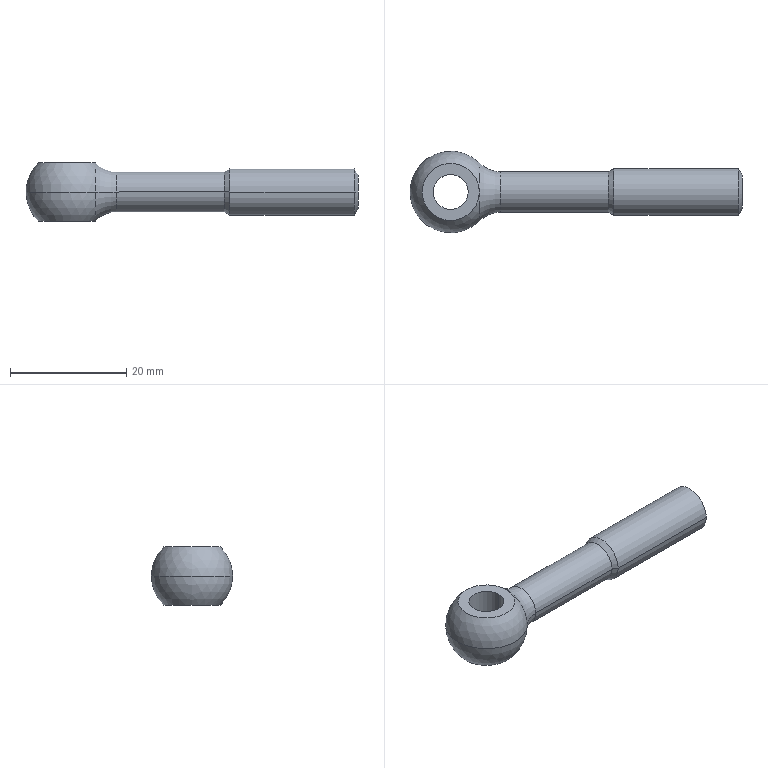Part | SolidWorks | features Cut 2, Revolution 2, Chamfer 1, Fillet 1, LPattern 1, RevCut 1 | 1 solid | 17 faces | box 57 x 14 x 10 mm | volume 2922 mm3 | cylinder 6 | cone 4 | plane 3 | torus 2 | sphere 2 | commonest cylinder face diameters 6 x2 6.918 x2 8 x2
STEP:
#1=CARTESIAN_POINT('',(4.965,4.934,0.));
#2=VERTEX_POINT('',#1);
#3=CARTESIAN_POINT('',(4.965,-4.934,0.));
#4=VERTEX_POINT('',#3);
#5=CARTESIAN_POINT('',(4.965,0.,0.));
#6=DIRECTION('',(-1.,0.,0.));
#7=DIRECTION('',(0.,-1.,0.));
#8=AXIS2_PLACEMENT_3D('',#5,#6,#7);
#9=CIRCLE('',#8,4.934);
#10=EDGE_CURVE('',#2,#4,#9,.T.);
#11=ORIENTED_EDGE('',*,*,#10,.F.);
#12=CARTESIAN_POINT('',(8.512,3.459,0.));
#13=VERTEX_POINT('',#12);
#14=CARTESIAN_POINT('',(8.512,8.459,0.));
#15=DIRECTION('',(0.,0.,1.));
#16=DIRECTION('',(0.,-1.,0.));
#17=AXIS2_PLACEMENT_3D('',#14,#15,#16);
#18=CIRCLE('',#17,5.);
#19=EDGE_CURVE('',#2,#13,#18,.T.);
#20=ORIENTED_EDGE('',*,*,#19,.T.);
#21=CARTESIAN_POINT('',(8.512,-3.459,0.));
#22=VERTEX_POINT('',#21);
#23=CARTESIAN_POINT('',(8.512,0.,0.));
#24=DIRECTION('',(1.,0.,0.));
#25=DIRECTION('',(0.,-1.,0.));
#26=AXIS2_PLACEMENT_3D('',#23,#24,#25);
#27=CIRCLE('',#26,3.459);
#28=EDGE_CURVE('',#22,#13,#27,.T.);
#29=ORIENTED_EDGE('',*,*,#28,.F.);
#30=CARTESIAN_POINT('',(8.512,-8.459,0.));
#31=DIRECTION('',(0.,0.,-1.));
#32=DIRECTION('',(-1.,0.,0.));
#33=AXIS2_PLACEMENT_3D('',#30,#31,#32);
#34=CIRCLE('',#33,5.);
#35=EDGE_CURVE('',#4,#22,#34,.T.);
#36=ORIENTED_EDGE('',*,*,#35,.F.);
#37=EDGE_LOOP('',(#11,#20,#29,#36));
#38=FACE_OUTER_BOUND('',#37,.T.);
#39=CARTESIAN_POINT('',(8.512,0.,0.));
#40=DIRECTION('',(-1.,0.,0.));
#41=DIRECTION('',(0.,-1.,0.));
#42=AXIS2_PLACEMENT_3D('',#39,#40,#41);
#43=TOROIDAL_SURFACE('',#42,8.459,5.);
#44=ADVANCED_FACE('',(#38),#43,.F.);
#45=CARTESIAN_POINT('',(50.,-2.918,0.));
#46=VERTEX_POINT('',#45);
#47=CARTESIAN_POINT('',(50.,2.917,0.));
#48=VERTEX_POINT('',#47);
#49=CARTESIAN_POINT('',(50.,0.,0.));
#50=DIRECTION('',(-1.,0.,0.));
#51=DIRECTION('',(0.,-1.,0.));
#52=AXIS2_PLACEMENT_3D('',#49,#50,#51);
#53=CIRCLE('',#52,2.918);
#54=EDGE_CURVE('',#46,#48,#53,.T.);
#55=ORIENTED_EDGE('',*,*,#54,.T.);
#56=CARTESIAN_POINT('',(49.375,4.,0.));
#57=VERTEX_POINT('',#56);
#58=CARTESIAN_POINT('',(49.375,4.,0.));
#59=DIRECTION('',(-0.5,0.866,0.));
#60=VECTOR('',#59,1000.);
#61=LINE('',#58,#60);
#62=EDGE_CURVE('',#48,#57,#61,.T.);
#63=ORIENTED_EDGE('',*,*,#62,.T.);
#64=CARTESIAN_POINT('',(49.375,-4.,0.));
#65=VERTEX_POINT('',#64);
#66=CARTESIAN_POINT('',(49.375,0.,0.));
#67=DIRECTION('',(-1.,0.,0.));
#68=DIRECTION('',(0.,-1.,0.));
#69=AXIS2_PLACEMENT_3D('',#66,#67,#68);
#70=CIRCLE('',#69,4.);
#71=EDGE_CURVE('',#65,#57,#70,.T.);
#72=ORIENTED_EDGE('',*,*,#71,.F.);
#73=CARTESIAN_POINT('',(49.375,-4.,0.));
#74=DIRECTION('',(-0.5,-0.866,0.));
#75=VECTOR('',#74,1000.);
#76=LINE('',#73,#75);
#77=EDGE_CURVE('',#46,#65,#76,.T.);
#78=ORIENTED_EDGE('',*,*,#77,.F.);
#79=EDGE_LOOP('',(#55,#63,#72,#78));
#80=FACE_OUTER_BOUND('',#79,.T.);
#81=CARTESIAN_POINT('',(49.375,0.,0.));
#82=DIRECTION('',(-1.,0.,0.));
#83=DIRECTION('',(0.,-1.,0.));
#84=AXIS2_PLACEMENT_3D('',#81,#82,#83);
#85=CONICAL_SURFACE('',#84,4.,1.047);
#86=ADVANCED_FACE('',(#80),#85,.T.);
#87=CARTESIAN_POINT('',(27.063,-3.459,0.));
#88=VERTEX_POINT('',#87);
#89=CARTESIAN_POINT('',(27.063,3.459,0.));
#90=VERTEX_POINT('',#89);
#91=CARTESIAN_POINT('',(27.063,0.,0.));
#92=DIRECTION('',(-1.,0.,0.));
#93=DIRECTION('',(0.,-1.,0.));
#94=AXIS2_PLACEMENT_3D('',#91,#92,#93);
#95=CIRCLE('',#94,3.459);
#96=EDGE_CURVE('',#88,#90,#95,.T.);
#97=ORIENTED_EDGE('',*,*,#96,.F.);
#98=CARTESIAN_POINT('',(28.,-4.,0.));
#99=VERTEX_POINT('',#98);
#100=CARTESIAN_POINT('',(28.,-4.,0.));
#101=DIRECTION('',(0.866,-0.5,0.));
#102=VECTOR('',#101,1000.);
#103=LINE('',#100,#102);
#104=EDGE_CURVE('',#88,#99,#103,.T.);
#105=ORIENTED_EDGE('',*,*,#104,.T.);
#106=CARTESIAN_POINT('',(28.,4.,0.));
#107=VERTEX_POINT('',#106);
#108=CARTESIAN_POINT('',(28.,0.,0.));
#109=DIRECTION('',(-1.,0.,0.));
#110=DIRECTION('',(0.,-1.,0.));
#111=AXIS2_PLACEMENT_3D('',#108,#109,#110);
#112=CIRCLE('',#111,4.);
#113=EDGE_CURVE('',#99,#107,#112,.T.);
#114=ORIENTED_EDGE('',*,*,#113,.T.);
#115=CARTESIAN_POINT('',(28.,4.,0.));
#116=DIRECTION('',(0.866,0.5,0.));
#117=VECTOR('',#116,1000.);
#118=LINE('',#115,#117);
#119=EDGE_CURVE('',#90,#107,#118,.T.);
#120=ORIENTED_EDGE('',*,*,#119,.F.);
#121=EDGE_LOOP('',(#97,#105,#114,#120));
#122=FACE_OUTER_BOUND('',#121,.T.);
#123=CARTESIAN_POINT('',(28.,0.,0.));
#124=DIRECTION('',(1.,0.,0.));
#125=DIRECTION('',(0.,1.,0.));
#126=AXIS2_PLACEMENT_3D('',#123,#124,#125);
#127=CONICAL_SURFACE('',#126,4.,0.5236);
#128=ADVANCED_FACE('',(#122),#127,.T.);
#129=ORIENTED_EDGE('',*,*,#96,.T.);
#130=CARTESIAN_POINT('',(0.,3.459,0.));
#131=DIRECTION('',(-1.,0.,0.));
#132=VECTOR('',#131,1000.);
#133=LINE('',#130,#132);
#134=EDGE_CURVE('',#90,#13,#133,.T.);
#135=ORIENTED_EDGE('',*,*,#134,.T.);
#136=CARTESIAN_POINT('',(8.512,0.,0.));
#137=DIRECTION('',(1.,0.,0.));
#138=DIRECTION('',(0.,-1.,0.));
#139=AXIS2_PLACEMENT_3D('',#136,#137,#138);
#140=CIRCLE('',#139,3.459);
#141=EDGE_CURVE('',#13,#22,#140,.T.);
#142=ORIENTED_EDGE('',*,*,#141,.T.);
#143=CARTESIAN_POINT('',(0.,-3.459,0.));
#144=DIRECTION('',(-1.,0.,0.));
#145=VECTOR('',#144,1000.);
#146=LINE('',#143,#145);
#147=EDGE_CURVE('',#88,#22,#146,.T.);
#148=ORIENTED_EDGE('',*,*,#147,.F.);
#149=EDGE_LOOP('',(#129,#135,#142,#148));
#150=FACE_OUTER_BOUND('',#149,.T.);
#151=CARTESIAN_POINT('',(0.,0.,0.));
#152=DIRECTION('',(-1.,0.,0.));
#153=DIRECTION('',(0.,-1.,0.));
#154=AXIS2_PLACEMENT_3D('',#151,#152,#153);
#155=CYLINDRICAL_SURFACE('',#154,3.459);
#156=ADVANCED_FACE('',(#150),#155,.T.);
#157=CARTESIAN_POINT('',(-3.,0.,-5.));
#158=VERTEX_POINT('',#157);
#159=CARTESIAN_POINT('',(3.,0.,-5.));
#160=VERTEX_POINT('',#159);
#161=CARTESIAN_POINT('',(0.,0.,-5.));
#162=DIRECTION('',(0.,0.,1.));
#163=DIRECTION('',(1.,0.,0.));
#164=AXIS2_PLACEMENT_3D('',#161,#162,#163);
#165=CIRCLE('',#164,3.);
#166=EDGE_CURVE('',#158,#160,#165,.T.);
#167=ORIENTED_EDGE('',*,*,#166,.F.);
#168=CARTESIAN_POINT('',(-3.,0.,5.));
#169=VERTEX_POINT('',#168);
#170=CARTESIAN_POINT('',(-3.,0.,-5.));
#171=DIRECTION('',(0.,0.,1.));
#172=VECTOR('',#171,1000.);
#173=LINE('',#170,#172);
#174=EDGE_CURVE('',#158,#169,#173,.T.);
#175=ORIENTED_EDGE('',*,*,#174,.T.);
#176=CARTESIAN_POINT('',(3.,0.,5.));
#177=VERTEX_POINT('',#176);
#178=CARTESIAN_POINT('',(0.,0.,5.));
#179=DIRECTION('',(0.,0.,1.));
#180=DIRECTION('',(1.,0.,0.));
#181=AXIS2_PLACEMENT_3D('',#178,#179,#180);
#182=CIRCLE('',#181,3.);
#183=EDGE_CURVE('',#169,#177,#182,.T.);
#184=ORIENTED_EDGE('',*,*,#183,.T.);
#185=CARTESIAN_POINT('',(3.,0.,-5.));
#186=DIRECTION('',(0.,0.,1.));
#187=VECTOR('',#186,1000.);
#188=LINE('',#185,#187);
#189=EDGE_CURVE('',#160,#177,#188,.T.);
#190=ORIENTED_EDGE('',*,*,#189,.F.);
#191=EDGE_LOOP('',(#167,#175,#184,#190));
#192=FACE_OUTER_BOUND('',#191,.T.);
#193=CARTESIAN_POINT('',(0.,0.,-5.));
#194=DIRECTION('',(0.,0.,1.));
#195=DIRECTION('',(1.,0.,0.));
#196=AXIS2_PLACEMENT_3D('',#193,#194,#195);
#197=CYLINDRICAL_SURFACE('',#196,3.);
#198=ADVANCED_FACE('',(#192),#197,.F.);
#199=CARTESIAN_POINT('',(4.899,0.,-5.));
#200=VERTEX_POINT('',#199);
#201=CARTESIAN_POINT('',(-4.899,0.,-5.));
#202=VERTEX_POINT('',#201);
#203=CARTESIAN_POINT('',(0.,0.,-5.));
#204=DIRECTION('',(0.,0.,1.));
#205=DIRECTION('',(1.,0.,0.));
#206=AXIS2_PLACEMENT_3D('',#203,#204,#205);
#207=CIRCLE('',#206,4.899);
#208=EDGE_CURVE('',#200,#202,#207,.T.);
#209=ORIENTED_EDGE('',*,*,#208,.T.);
#210=CARTESIAN_POINT('',(0.,0.,-5.));
#211=DIRECTION('',(0.,0.,1.));
#212=DIRECTION('',(1.,0.,0.));
#213=AXIS2_PLACEMENT_3D('',#210,#211,#212);
#214=CIRCLE('',#213,4.899);
#215=EDGE_CURVE('',#202,#200,#214,.T.);
#216=ORIENTED_EDGE('',*,*,#215,.T.);
#217=EDGE_LOOP('',(#209,#216));
#218=FACE_BOUND('',#217,.T.);
#219=ORIENTED_EDGE('',*,*,#10,.T.);
#220=CARTESIAN_POINT('',(-7.,0.,0.));
#221=VERTEX_POINT('',#220);
#222=CARTESIAN_POINT('',(0.,0.,0.));
#223=DIRECTION('',(0.,0.,-1.));
#224=DIRECTION('',(0.,1.,0.));
#225=AXIS2_PLACEMENT_3D('',#222,#223,#224);
#226=CIRCLE('',#225,7.);
#227=EDGE_CURVE('',#4,#221,#226,.T.);
#228=ORIENTED_EDGE('',*,*,#227,.T.);
#229=CARTESIAN_POINT('',(0.,0.,0.));
#230=DIRECTION('',(0.,0.,1.));
#231=DIRECTION('',(1.,0.,0.));
#232=AXIS2_PLACEMENT_3D('',#229,#230,#231);
#233=CIRCLE('',#232,7.);
#234=EDGE_CURVE('',#2,#221,#233,.T.);
#235=ORIENTED_EDGE('',*,*,#234,.F.);
#236=EDGE_LOOP('',(#219,#228,#235));
#237=FACE_OUTER_BOUND('',#236,.T.);
#238=CARTESIAN_POINT('',(0.,0.,0.));
#239=DIRECTION('',(0.,0.,-1.));
#240=DIRECTION('',(0.,1.,0.));
#241=AXIS2_PLACEMENT_3D('',#238,#239,#240);
#242=SPHERICAL_SURFACE('',#241,7.);
#243=ADVANCED_FACE('',(#218,#237),#242,.T.);
#244=ORIENTED_EDGE('',*,*,#71,.T.);
#245=CARTESIAN_POINT('',(0.,4.,0.));
#246=DIRECTION('',(-1.,0.,0.));
#247=VECTOR('',#246,1000.);
#248=LINE('',#245,#247);
#249=EDGE_CURVE('',#57,#107,#248,.T.);
#250=ORIENTED_EDGE('',*,*,#249,.T.);
#251=ORIENTED_EDGE('',*,*,#113,.F.);
#252=CARTESIAN_POINT('',(0.,-4.,0.));
#253=DIRECTION('',(-1.,0.,0.));
#254=VECTOR('',#253,1000.);
#255=LINE('',#252,#254);
#256=EDGE_CURVE('',#65,#99,#255,.T.);
#257=ORIENTED_EDGE('',*,*,#256,.F.);
#258=EDGE_LOOP('',(#244,#250,#251,#257));
#259=FACE_OUTER_BOUND('',#258,.T.);
#260=CARTESIAN_POINT('',(0.,0.,0.));
#261=DIRECTION('',(-1.,0.,0.));
#262=DIRECTION('',(0.,-1.,0.));
#263=AXIS2_PLACEMENT_3D('',#260,#261,#262);
#264=CYLINDRICAL_SURFACE('',#263,4.);
#265=ADVANCED_FACE('',(#259),#264,.T.);
#266=ORIENTED_EDGE('',*,*,#249,.F.);
#267=CARTESIAN_POINT('',(49.375,0.,0.));
#268=DIRECTION('',(-1.,0.,0.));
#269=DIRECTION('',(0.,-1.,0.));
#270=AXIS2_PLACEMENT_3D('',#267,#268,#269);
#271=CIRCLE('',#270,4.);
#272=EDGE_CURVE('',#57,#65,#271,.T.);
#273=ORIENTED_EDGE('',*,*,#272,.T.);
#274=ORIENTED_EDGE('',*,*,#256,.T.);
#275=CARTESIAN_POINT('',(28.,0.,0.));
#276=DIRECTION('',(-1.,0.,0.));
#277=DIRECTION('',(0.,-1.,0.));
#278=AXIS2_PLACEMENT_3D('',#275,#276,#277);
#279=CIRCLE('',#278,4.);
#280=EDGE_CURVE('',#107,#99,#279,.T.);
#281=ORIENTED_EDGE('',*,*,#280,.F.);
#282=EDGE_LOOP('',(#266,#273,#274,#281));
#283=FACE_OUTER_BOUND('',#282,.T.);
#284=CARTESIAN_POINT('',(0.,0.,0.));
#285=DIRECTION('',(-1.,0.,0.));
#286=DIRECTION('',(0.,-1.,0.));
#287=AXIS2_PLACEMENT_3D('',#284,#285,#286);
#288=CYLINDRICAL_SURFACE('',#287,4.);
#289=ADVANCED_FACE('',(#283),#288,.T.);
#290=ORIENTED_EDGE('',*,*,#227,.F.);
#291=CARTESIAN_POINT('',(4.965,0.,0.));
#292=DIRECTION('',(-1.,0.,0.));
#293=DIRECTION('',(0.,-1.,0.));
#294=AXIS2_PLACEMENT_3D('',#291,#292,#293);
#295=CIRCLE('',#294,4.934);
#296=EDGE_CURVE('',#4,#2,#295,.T.);
#297=ORIENTED_EDGE('',*,*,#296,.T.);
#298=ORIENTED_EDGE('',*,*,#234,.T.);
#299=EDGE_LOOP('',(#290,#297,#298));
#300=FACE_OUTER_BOUND('',#299,.T.);
#301=CARTESIAN_POINT('',(-4.899,0.,5.));
#302=VERTEX_POINT('',#301);
#303=CARTESIAN_POINT('',(4.899,0.,5.));
#304=VERTEX_POINT('',#303);
#305=CARTESIAN_POINT('',(0.,0.,5.));
#306=DIRECTION('',(0.,0.,-1.));
#307=DIRECTION('',(-1.,0.,0.));
#308=AXIS2_PLACEMENT_3D('',#305,#306,#307);
#309=CIRCLE('',#308,4.899);
#310=EDGE_CURVE('',#302,#304,#309,.T.);
#311=ORIENTED_EDGE('',*,*,#310,.T.);
#312=CARTESIAN_POINT('',(0.,0.,5.));
#313=DIRECTION('',(0.,0.,-1.));
#314=DIRECTION('',(-1.,0.,0.));
#315=AXIS2_PLACEMENT_3D('',#312,#313,#314);
#316=CIRCLE('',#315,4.899);
#317=EDGE_CURVE('',#304,#302,#316,.T.);
#318=ORIENTED_EDGE('',*,*,#317,.T.);
#319=EDGE_LOOP('',(#311,#318));
#320=FACE_BOUND('',#319,.T.);
#321=CARTESIAN_POINT('',(0.,0.,0.));
#322=DIRECTION('',(0.,0.,-1.));
#323=DIRECTION('',(0.,1.,0.));
#324=AXIS2_PLACEMENT_3D('',#321,#322,#323);
#325=SPHERICAL_SURFACE('',#324,7.);
#326=ADVANCED_FACE('',(#300,#320),#325,.T.);
#327=CARTESIAN_POINT('',(0.,0.,5.));
#328=DIRECTION('',(0.,0.,1.));
#329=DIRECTION('',(1.,0.,0.));
#330=AXIS2_PLACEMENT_3D('',#327,#328,#329);
#331=CIRCLE('',#330,3.);
#332=EDGE_CURVE('',#177,#169,#331,.T.);
#333=ORIENTED_EDGE('',*,*,#332,.F.);
#334=ORIENTED_EDGE('',*,*,#183,.F.);
#335=EDGE_LOOP('',(#333,#334));
#336=FACE_BOUND('',#335,.T.);
#337=ORIENTED_EDGE('',*,*,#310,.F.);
#338=ORIENTED_EDGE('',*,*,#317,.F.);
#339=EDGE_LOOP('',(#337,#338));
#340=FACE_OUTER_BOUND('',#339,.T.);
#341=CARTESIAN_POINT('',(-7.,4.899,5.));
#342=DIRECTION('',(0.,0.,-1.));
#343=DIRECTION('',(-1.,0.,0.));
#344=AXIS2_PLACEMENT_3D('',#341,#342,#343);
#345=PLANE('',#344);
#346=ADVANCED_FACE('',(#336,#340),#345,.F.);
#347=CARTESIAN_POINT('',(0.,0.,-5.));
#348=DIRECTION('',(0.,0.,1.));
#349=DIRECTION('',(1.,0.,0.));
#350=AXIS2_PLACEMENT_3D('',#347,#348,#349);
#351=CIRCLE('',#350,3.);
#352=EDGE_CURVE('',#160,#158,#351,.T.);
#353=ORIENTED_EDGE('',*,*,#352,.T.);
#354=ORIENTED_EDGE('',*,*,#166,.T.);
#355=EDGE_LOOP('',(#353,#354));
#356=FACE_BOUND('',#355,.T.);
#357=ORIENTED_EDGE('',*,*,#208,.F.);
#358=ORIENTED_EDGE('',*,*,#215,.F.);
#359=EDGE_LOOP('',(#357,#358));
#360=FACE_OUTER_BOUND('',#359,.T.);
#361=CARTESIAN_POINT('',(-7.,4.899,-5.));
#362=DIRECTION('',(0.,0.,1.));
#363=DIRECTION('',(1.,0.,0.));
#364=AXIS2_PLACEMENT_3D('',#361,#362,#363);
#365=PLANE('',#364);
#366=ADVANCED_FACE('',(#356,#360),#365,.F.);
#367=ORIENTED_EDGE('',*,*,#174,.F.);
#368=ORIENTED_EDGE('',*,*,#352,.F.);
#369=ORIENTED_EDGE('',*,*,#189,.T.);
#370=ORIENTED_EDGE('',*,*,#332,.T.);
#371=EDGE_LOOP('',(#367,#368,#369,#370));
#372=FACE_OUTER_BOUND('',#371,.T.);
#373=CARTESIAN_POINT('',(0.,0.,-5.));
#374=DIRECTION('',(0.,0.,1.));
#375=DIRECTION('',(1.,0.,0.));
#376=AXIS2_PLACEMENT_3D('',#373,#374,#375);
#377=CYLINDRICAL_SURFACE('',#376,3.);
#378=ADVANCED_FACE('',(#372),#377,.F.);
#379=ORIENTED_EDGE('',*,*,#134,.F.);
#380=CARTESIAN_POINT('',(27.063,0.,0.));
#381=DIRECTION('',(-1.,0.,0.));
#382=DIRECTION('',(0.,-1.,0.));
#383=AXIS2_PLACEMENT_3D('',#380,#381,#382);
#384=CIRCLE('',#383,3.459);
#385=EDGE_CURVE('',#90,#88,#384,.T.);
#386=ORIENTED_EDGE('',*,*,#385,.T.);
#387=ORIENTED_EDGE('',*,*,#147,.T.);
#388=ORIENTED_EDGE('',*,*,#28,.T.);
#389=EDGE_LOOP('',(#379,#386,#387,#388));
#390=FACE_OUTER_BOUND('',#389,.T.);
#391=CARTESIAN_POINT('',(0.,0.,0.));
#392=DIRECTION('',(-1.,0.,0.));
#393=DIRECTION('',(0.,-1.,0.));
#394=AXIS2_PLACEMENT_3D('',#391,#392,#393);
#395=CYLINDRICAL_SURFACE('',#394,3.459);
#396=ADVANCED_FACE('',(#390),#395,.T.);
#397=ORIENTED_EDGE('',*,*,#104,.F.);
#398=ORIENTED_EDGE('',*,*,#385,.F.);
#399=ORIENTED_EDGE('',*,*,#119,.T.);
#400=ORIENTED_EDGE('',*,*,#280,.T.);
#401=EDGE_LOOP('',(#397,#398,#399,#400));
#402=FACE_OUTER_BOUND('',#401,.T.);
#403=CARTESIAN_POINT('',(28.,0.,0.));
#404=DIRECTION('',(1.,0.,0.));
#405=DIRECTION('',(0.,1.,0.));
#406=AXIS2_PLACEMENT_3D('',#403,#404,#405);
#407=CONICAL_SURFACE('',#406,4.,0.5236);
#408=ADVANCED_FACE('',(#402),#407,.T.);
#409=ORIENTED_EDGE('',*,*,#62,.F.);
#410=CARTESIAN_POINT('',(50.,0.,0.));
#411=DIRECTION('',(-1.,0.,0.));
#412=DIRECTION('',(0.,-1.,0.));
#413=AXIS2_PLACEMENT_3D('',#410,#411,#412);
#414=CIRCLE('',#413,2.918);
#415=EDGE_CURVE('',#48,#46,#414,.T.);
#416=ORIENTED_EDGE('',*,*,#415,.T.);
#417=ORIENTED_EDGE('',*,*,#77,.T.);
#418=ORIENTED_EDGE('',*,*,#272,.F.);
#419=EDGE_LOOP('',(#409,#416,#417,#418));
#420=FACE_OUTER_BOUND('',#419,.T.);
#421=CARTESIAN_POINT('',(49.375,0.,0.));
#422=DIRECTION('',(-1.,0.,0.));
#423=DIRECTION('',(0.,-1.,0.));
#424=AXIS2_PLACEMENT_3D('',#421,#422,#423);
#425=CONICAL_SURFACE('',#424,4.,1.047);
#426=ADVANCED_FACE('',(#420),#425,.T.);
#427=ORIENTED_EDGE('',*,*,#54,.F.);
#428=ORIENTED_EDGE('',*,*,#415,.F.);
#429=EDGE_LOOP('',(#427,#428));
#430=FACE_OUTER_BOUND('',#429,.T.);
#431=CARTESIAN_POINT('',(50.,4.,0.));
#432=DIRECTION('',(-1.,0.,0.));
#433=DIRECTION('',(0.,-1.,0.));
#434=AXIS2_PLACEMENT_3D('',#431,#432,#433);
#435=PLANE('',#434);
#436=ADVANCED_FACE('',(#430),#435,.F.);
#437=ORIENTED_EDGE('',*,*,#19,.F.);
#438=ORIENTED_EDGE('',*,*,#296,.F.);
#439=ORIENTED_EDGE('',*,*,#35,.T.);
#440=ORIENTED_EDGE('',*,*,#141,.F.);
#441=EDGE_LOOP('',(#437,#438,#439,#440));
#442=FACE_OUTER_BOUND('',#441,.T.);
#443=CARTESIAN_POINT('',(8.512,0.,0.));
#444=DIRECTION('',(-1.,0.,0.));
#445=DIRECTION('',(0.,-1.,0.));
#446=AXIS2_PLACEMENT_3D('',#443,#444,#445);
#447=TOROIDAL_SURFACE('',#446,8.459,5.);
#448=ADVANCED_FACE('',(#442),#447,.F.);
#449=CLOSED_SHELL('',(#44,#86,#128,#156,#198,#243,#265,#289,#326,#346,#366,#378,#396,#408,#426,#436,#448));
#450=MANIFOLD_SOLID_BREP('',#449);
#451=CARTESIAN_POINT('',(0.,0.,0.));
#452=DIRECTION('',(0.,0.,1.));
#453=DIRECTION('',(1.,0.,0.));
#454=AXIS2_PLACEMENT_3D('',#451,#452,#453);
#455=(LENGTH_UNIT()NAMED_UNIT(*)SI_UNIT(.MILLI.,.METRE.));
#456=UNCERTAINTY_MEASURE_WITH_UNIT(LENGTH_MEASURE(0.00001),#455,'','');
#457=(NAMED_UNIT(*)PLANE_ANGLE_UNIT()SI_UNIT($,.RADIAN.));
#458=(NAMED_UNIT(*)SI_UNIT($,.STERADIAN.)SOLID_ANGLE_UNIT());
#459=(GEOMETRIC_REPRESENTATION_CONTEXT(3)GLOBAL_UNCERTAINTY_ASSIGNED_CONTEXT((#456))GLOBAL_UNIT_ASSIGNED_CONTEXT((#455,#457,#458))REPRESENTATION_CONTEXT('',''));
#460=ADVANCED_BREP_SHAPE_REPRESENTATION('',(#450,#454),#459);